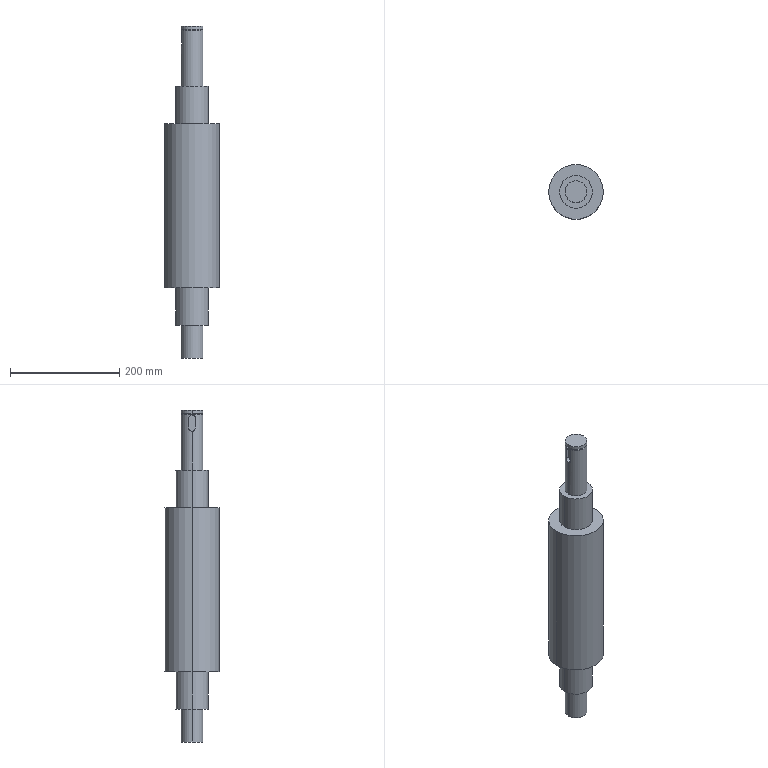Part | STEP file | 1 solid | 28 faces | box 100 x 100 x 607 mm | volume 2954002 mm3 | cylinder 17 | plane 11 | commonest cylinder face diameters 40 x6 60 x4 12 x3 33 x2 100 x2